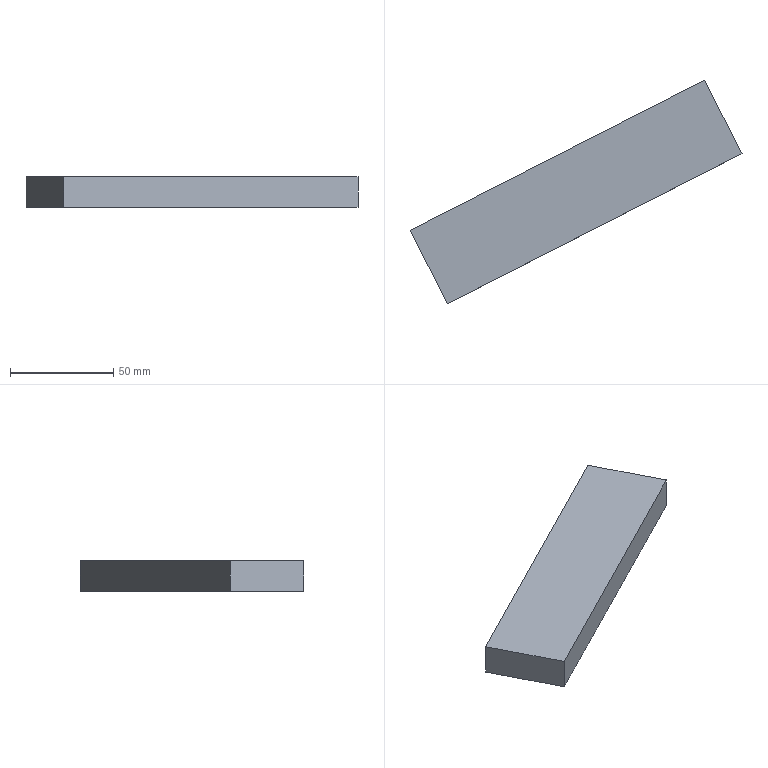Part | NX | features solid 2 | 1 solid | 6 faces | box 160.721 x 108.279 x 15 mm | volume 96000 mm3 | plane 6
STEP:
#1=CARTESIAN_POINT('',(-1572.22,-383.581,165.));
#2=VERTEX_POINT('',#1);
#3=CARTESIAN_POINT('',(-1572.22,-383.581,180.));
#4=VERTEX_POINT('',#3);
#5=CARTESIAN_POINT('',(-1572.22,-383.581,165.));
#6=DIRECTION('',(0.,0.,1.));
#7=VECTOR('',#6,1000.);
#8=LINE('',#5,#7);
#9=EDGE_CURVE('',#2,#4,#8,.T.);
#10=ORIENTED_EDGE('',*,*,#9,.T.);
#11=CARTESIAN_POINT('',(-1714.781,-456.219,180.));
#12=VERTEX_POINT('',#11);
#13=CARTESIAN_POINT('',(-1714.781,-456.219,180.));
#14=DIRECTION('',(0.891,0.454,0.));
#15=VECTOR('',#14,1000.);
#16=LINE('',#13,#15);
#17=EDGE_CURVE('',#12,#4,#16,.T.);
#18=ORIENTED_EDGE('',*,*,#17,.F.);
#19=CARTESIAN_POINT('',(-1714.781,-456.219,165.));
#20=VERTEX_POINT('',#19);
#21=CARTESIAN_POINT('',(-1714.781,-456.219,165.));
#22=DIRECTION('',(0.,0.,1.));
#23=VECTOR('',#22,1000.);
#24=LINE('',#21,#23);
#25=EDGE_CURVE('',#20,#12,#24,.T.);
#26=ORIENTED_EDGE('',*,*,#25,.F.);
#27=CARTESIAN_POINT('',(-1714.781,-456.219,165.));
#28=DIRECTION('',(0.891,0.454,0.));
#29=VECTOR('',#28,1000.);
#30=LINE('',#27,#29);
#31=EDGE_CURVE('',#20,#2,#30,.T.);
#32=ORIENTED_EDGE('',*,*,#31,.T.);
#33=EDGE_LOOP('',(#10,#18,#26,#32));
#34=FACE_BOUND('',#33,.T.);
#35=CARTESIAN_POINT('',(-1714.781,-456.219,165.));
#36=DIRECTION('',(0.454,-0.891,0.));
#37=DIRECTION('',(0.,0.,1.));
#38=AXIS2_PLACEMENT_3D('',#35,#36,#37);
#39=PLANE('',#38);
#40=ADVANCED_FACE('',(#34),#39,.T.);
#41=CARTESIAN_POINT('',(-1590.379,-347.94,180.));
#42=VERTEX_POINT('',#41);
#43=CARTESIAN_POINT('',(-1572.22,-383.581,180.));
#44=DIRECTION('',(-0.454,0.891,0.));
#45=VECTOR('',#44,1000.);
#46=LINE('',#43,#45);
#47=EDGE_CURVE('',#4,#42,#46,.T.);
#48=ORIENTED_EDGE('',*,*,#47,.T.);
#49=CARTESIAN_POINT('',(-1732.94,-420.579,180.));
#50=VERTEX_POINT('',#49);
#51=CARTESIAN_POINT('',(-1732.94,-420.579,180.));
#52=DIRECTION('',(0.891,0.454,0.));
#53=VECTOR('',#52,1000.);
#54=LINE('',#51,#53);
#55=EDGE_CURVE('',#50,#42,#54,.T.);
#56=ORIENTED_EDGE('',*,*,#55,.F.);
#57=CARTESIAN_POINT('',(-1714.781,-456.219,180.));
#58=DIRECTION('',(-0.454,0.891,0.));
#59=VECTOR('',#58,1000.);
#60=LINE('',#57,#59);
#61=EDGE_CURVE('',#12,#50,#60,.T.);
#62=ORIENTED_EDGE('',*,*,#61,.F.);
#63=ORIENTED_EDGE('',*,*,#17,.T.);
#64=EDGE_LOOP('',(#48,#56,#62,#63));
#65=FACE_BOUND('',#64,.T.);
#66=CARTESIAN_POINT('',(-1714.781,-456.219,180.));
#67=DIRECTION('',(0.,0.,1.));
#68=DIRECTION('',(0.891,0.454,0.));
#69=AXIS2_PLACEMENT_3D('',#66,#67,#68);
#70=PLANE('',#69);
#71=ADVANCED_FACE('',(#65),#70,.T.);
#72=CARTESIAN_POINT('',(-1590.379,-347.94,165.));
#73=VERTEX_POINT('',#72);
#74=CARTESIAN_POINT('',(-1590.379,-347.94,180.));
#75=DIRECTION('',(0.,0.,-1.));
#76=VECTOR('',#75,1000.);
#77=LINE('',#74,#76);
#78=EDGE_CURVE('',#42,#73,#77,.T.);
#79=ORIENTED_EDGE('',*,*,#78,.T.);
#80=CARTESIAN_POINT('',(-1732.94,-420.579,165.));
#81=VERTEX_POINT('',#80);
#82=CARTESIAN_POINT('',(-1732.94,-420.579,165.));
#83=DIRECTION('',(0.891,0.454,0.));
#84=VECTOR('',#83,1000.);
#85=LINE('',#82,#84);
#86=EDGE_CURVE('',#81,#73,#85,.T.);
#87=ORIENTED_EDGE('',*,*,#86,.F.);
#88=CARTESIAN_POINT('',(-1732.94,-420.579,180.));
#89=DIRECTION('',(0.,0.,-1.));
#90=VECTOR('',#89,1000.);
#91=LINE('',#88,#90);
#92=EDGE_CURVE('',#50,#81,#91,.T.);
#93=ORIENTED_EDGE('',*,*,#92,.F.);
#94=ORIENTED_EDGE('',*,*,#55,.T.);
#95=EDGE_LOOP('',(#79,#87,#93,#94));
#96=FACE_BOUND('',#95,.T.);
#97=CARTESIAN_POINT('',(-1732.94,-420.579,180.));
#98=DIRECTION('',(-0.454,0.891,0.));
#99=DIRECTION('',(0.,0.,-1.));
#100=AXIS2_PLACEMENT_3D('',#97,#98,#99);
#101=PLANE('',#100);
#102=ADVANCED_FACE('',(#96),#101,.T.);
#103=CARTESIAN_POINT('',(-1572.22,-383.581,165.));
#104=DIRECTION('',(-0.454,0.891,0.));
#105=VECTOR('',#104,1000.);
#106=LINE('',#103,#105);
#107=EDGE_CURVE('',#2,#73,#106,.T.);
#108=ORIENTED_EDGE('',*,*,#107,.F.);
#109=ORIENTED_EDGE('',*,*,#31,.F.);
#110=CARTESIAN_POINT('',(-1714.781,-456.219,165.));
#111=DIRECTION('',(-0.454,0.891,0.));
#112=VECTOR('',#111,1000.);
#113=LINE('',#110,#112);
#114=EDGE_CURVE('',#20,#81,#113,.T.);
#115=ORIENTED_EDGE('',*,*,#114,.T.);
#116=ORIENTED_EDGE('',*,*,#86,.T.);
#117=EDGE_LOOP('',(#108,#109,#115,#116));
#118=FACE_BOUND('',#117,.T.);
#119=CARTESIAN_POINT('',(-1714.781,-456.219,165.));
#120=DIRECTION('',(0.,0.,1.));
#121=DIRECTION('',(0.891,0.454,0.));
#122=AXIS2_PLACEMENT_3D('',#119,#120,#121);
#123=PLANE('',#122);
#124=ADVANCED_FACE('',(#118),#123,.F.);
#125=ORIENTED_EDGE('',*,*,#25,.T.);
#126=ORIENTED_EDGE('',*,*,#61,.T.);
#127=ORIENTED_EDGE('',*,*,#92,.T.);
#128=ORIENTED_EDGE('',*,*,#114,.F.);
#129=EDGE_LOOP('',(#125,#126,#127,#128));
#130=FACE_BOUND('',#129,.T.);
#131=CARTESIAN_POINT('',(-1714.781,-456.219,180.));
#132=DIRECTION('',(0.891,0.454,0.));
#133=DIRECTION('',(0.,0.,-1.));
#134=AXIS2_PLACEMENT_3D('',#131,#132,#133);
#135=PLANE('',#134);
#136=ADVANCED_FACE('',(#130),#135,.F.);
#137=ORIENTED_EDGE('',*,*,#9,.F.);
#138=ORIENTED_EDGE('',*,*,#107,.T.);
#139=ORIENTED_EDGE('',*,*,#78,.F.);
#140=ORIENTED_EDGE('',*,*,#47,.F.);
#141=EDGE_LOOP('',(#137,#138,#139,#140));
#142=FACE_BOUND('',#141,.T.);
#143=CARTESIAN_POINT('',(-1572.22,-383.581,180.));
#144=DIRECTION('',(0.891,0.454,0.));
#145=DIRECTION('',(0.,0.,-1.));
#146=AXIS2_PLACEMENT_3D('',#143,#144,#145);
#147=PLANE('',#146);
#148=ADVANCED_FACE('',(#142),#147,.T.);
#149=CLOSED_SHELL('',(#40,#71,#102,#124,#136,#148));
#150=MANIFOLD_SOLID_BREP('',#149);
#151=(LENGTH_UNIT()NAMED_UNIT(*)SI_UNIT(.MILLI.,.METRE.));
#152=UNCERTAINTY_MEASURE_WITH_UNIT(LENGTH_MEASURE(0.00001),#151,'','');
#153=(NAMED_UNIT(*)PLANE_ANGLE_UNIT()SI_UNIT($,.RADIAN.));
#154=(NAMED_UNIT(*)SI_UNIT($,.STERADIAN.)SOLID_ANGLE_UNIT());
#155=(GEOMETRIC_REPRESENTATION_CONTEXT(3)GLOBAL_UNCERTAINTY_ASSIGNED_CONTEXT((#152))GLOBAL_UNIT_ASSIGNED_CONTEXT((#151,#153,#154))REPRESENTATION_CONTEXT('',''));
#156=ADVANCED_BREP_SHAPE_REPRESENTATION('',(#150),#155);